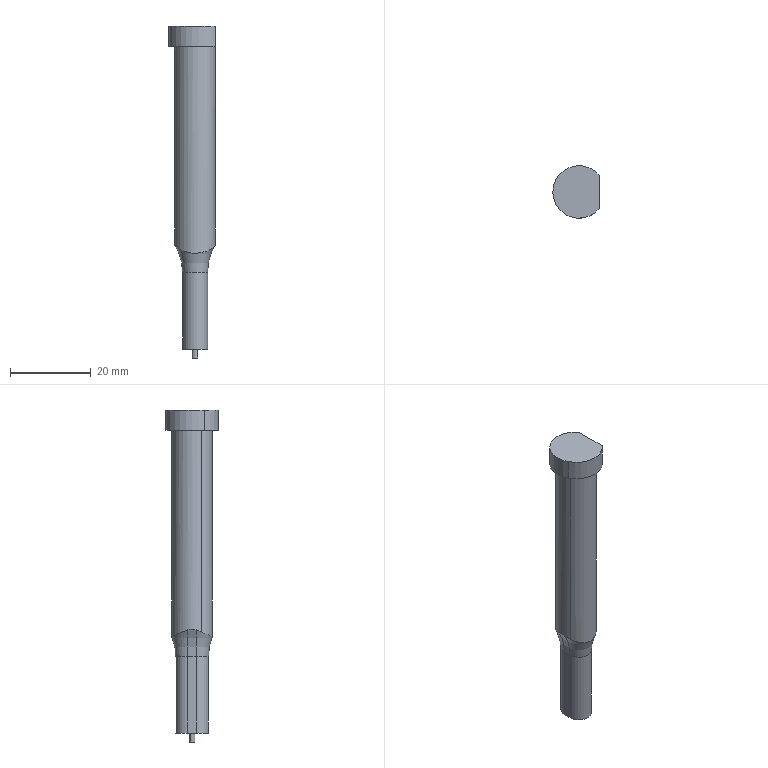Part | CATIA | 1 solid | 19 faces | box 11.5 x 13 x 82.2 mm | volume 5687 mm3 | cylinder 10 | plane 7 | torus 2 | commonest cylinder face diameters 1.47 x2 6.2 x2 10 x2 13 x2 26 x2
STEP:
#1=CARTESIAN_POINT('',(3.1,1.,0.));
#2=VERTEX_POINT('',#1);
#3=CARTESIAN_POINT('',(-3.1,1.,0.));
#4=VERTEX_POINT('',#3);
#5=CARTESIAN_POINT('',(0.,1.,0.));
#6=DIRECTION('',(0.,0.,1.));
#7=AXIS2_PLACEMENT_3D('',#5,#6,$);
#8=CIRCLE('',#7,3.1);
#9=EDGE_CURVE('',#2,#4,#8,.T.);
#10=ORIENTED_EDGE('',*,*,#9,.F.);
#11=CARTESIAN_POINT('',(3.1,-1.,0.));
#12=VERTEX_POINT('',#11);
#13=CARTESIAN_POINT('',(3.1,0.,0.));
#14=DIRECTION('',(0.,-1.,0.));
#15=VECTOR('',#14,1.);
#16=LINE('',#13,#15);
#17=EDGE_CURVE('',#2,#12,#16,.T.);
#18=ORIENTED_EDGE('',*,*,#17,.T.);
#19=CARTESIAN_POINT('',(-3.1,-1.,0.));
#20=VERTEX_POINT('',#19);
#21=CARTESIAN_POINT('',(0.,-1.,0.));
#22=DIRECTION('',(0.,0.,1.));
#23=AXIS2_PLACEMENT_3D('',#21,#22,$);
#24=CIRCLE('',#23,3.1);
#25=EDGE_CURVE('',#20,#12,#24,.T.);
#26=ORIENTED_EDGE('',*,*,#25,.F.);
#27=CARTESIAN_POINT('',(-3.1,0.,0.));
#28=DIRECTION('',(0.,1.,0.));
#29=VECTOR('',#28,1.);
#30=LINE('',#27,#29);
#31=EDGE_CURVE('',#20,#4,#30,.T.);
#32=ORIENTED_EDGE('',*,*,#31,.T.);
#33=EDGE_LOOP('',(#10,#18,#26,#32));
#34=FACE_OUTER_BOUND('',#33,.T.);
#35=CARTESIAN_POINT('',(0.645,-0.3524,0.));
#36=VERTEX_POINT('',#35);
#37=CARTESIAN_POINT('',(-0.645,0.3524,0.));
#38=VERTEX_POINT('',#37);
#39=CARTESIAN_POINT('',(0.,0.,0.));
#40=DIRECTION('',(0.,0.,1.));
#41=AXIS2_PLACEMENT_3D('',#39,#40,$);
#42=CIRCLE('',#41,0.735);
#43=EDGE_CURVE('',#36,#38,#42,.F.);
#44=ORIENTED_EDGE('',*,*,#43,.F.);
#45=CARTESIAN_POINT('',(0.,0.,0.));
#46=DIRECTION('',(0.,0.,1.));
#47=AXIS2_PLACEMENT_3D('',#45,#46,$);
#48=CIRCLE('',#47,0.735);
#49=EDGE_CURVE('',#38,#36,#48,.F.);
#50=ORIENTED_EDGE('',*,*,#49,.F.);
#51=EDGE_LOOP('',(#44,#50));
#52=FACE_BOUND('',#51,.T.);
#53=CARTESIAN_POINT('',(5.,0.,0.));
#54=DIRECTION('',(0.,0.,1.));
#55=DIRECTION('',(1.,0.,0.));
#56=AXIS2_PLACEMENT_3D('',#53,#54,#55);
#57=PLANE('',#56);
#58=ADVANCED_FACE('',(#34,#52),#57,.F.);
#59=CARTESIAN_POINT('',(4.388,2.397,25.072));
#60=VERTEX_POINT('',#59);
#61=CARTESIAN_POINT('',(4.899,1.,25.598));
#62=VERTEX_POINT('',#61);
#63=CARTESIAN_POINT('',(4.388,2.397,25.072));
#64=CARTESIAN_POINT('',(4.62,1.973,25.246));
#65=CARTESIAN_POINT('',(4.797,1.502,25.424));
#66=CARTESIAN_POINT('',(4.899,1.,25.598));
#67=B_SPLINE_CURVE_WITH_KNOTS('',3,(#63,#64,#65,#66),.UNSPECIFIED.,.F.,.U.,(4,4),(0.,5.244),.UNSPECIFIED.);
#68=EDGE_CURVE('',#60,#62,#67,.T.);
#69=ORIENTED_EDGE('',*,*,#68,.F.);
#70=CARTESIAN_POINT('',(4.388,2.397,75.));
#71=VERTEX_POINT('',#70);
#72=CARTESIAN_POINT('',(4.388,2.397,37.5));
#73=DIRECTION('',(0.,0.,1.));
#74=VECTOR('',#73,1.);
#75=LINE('',#72,#74);
#76=EDGE_CURVE('',#60,#71,#75,.T.);
#77=ORIENTED_EDGE('',*,*,#76,.T.);
#78=CARTESIAN_POINT('',(5.,0.,75.));
#79=VERTEX_POINT('',#78);
#80=CARTESIAN_POINT('',(0.,0.,75.));
#81=DIRECTION('',(0.,0.,1.));
#82=AXIS2_PLACEMENT_3D('',#80,#81,$);
#83=CIRCLE('',#82,5.);
#84=EDGE_CURVE('',#79,#71,#83,.T.);
#85=ORIENTED_EDGE('',*,*,#84,.F.);
#86=CARTESIAN_POINT('',(-4.388,-2.397,75.));
#87=VERTEX_POINT('',#86);
#88=CARTESIAN_POINT('',(0.,0.,75.));
#89=DIRECTION('',(0.,0.,1.));
#90=AXIS2_PLACEMENT_3D('',#88,#89,$);
#91=CIRCLE('',#90,5.);
#92=EDGE_CURVE('',#87,#79,#91,.T.);
#93=ORIENTED_EDGE('',*,*,#92,.F.);
#94=CARTESIAN_POINT('',(-4.388,-2.397,25.072));
#95=VERTEX_POINT('',#94);
#96=CARTESIAN_POINT('',(-4.388,-2.397,37.5));
#97=DIRECTION('',(0.,0.,1.));
#98=VECTOR('',#97,1.);
#99=LINE('',#96,#98);
#100=EDGE_CURVE('',#95,#87,#99,.T.);
#101=ORIENTED_EDGE('',*,*,#100,.F.);
#102=CARTESIAN_POINT('',(4.899,-1.,25.598));
#103=VERTEX_POINT('',#102);
#104=CARTESIAN_POINT('',(-4.388,-2.397,25.072));
#105=CARTESIAN_POINT('',(-4.106,-2.913,24.86));
#106=CARTESIAN_POINT('',(-3.757,-3.372,24.653));
#107=CARTESIAN_POINT('',(-3.357,-3.766,24.458));
#108=CARTESIAN_POINT('',(-2.497,-4.411,24.115));
#109=CARTESIAN_POINT('',(-1.535,-4.798,23.881));
#110=CARTESIAN_POINT('',(-1.049,-4.927,23.8));
#111=CARTESIAN_POINT('',(0.1474,-5.089,23.696));
#112=CARTESIAN_POINT('',(1.346,-4.893,23.821));
#113=CARTESIAN_POINT('',(2.03,-4.655,23.973));
#114=CARTESIAN_POINT('',(3.209,-3.988,24.358));
#115=CARTESIAN_POINT('',(4.144,-2.909,24.867));
#116=CARTESIAN_POINT('',(4.498,-2.338,25.111));
#117=CARTESIAN_POINT('',(4.757,-1.693,25.358));
#118=CARTESIAN_POINT('',(4.899,-1.,25.598));
#119=B_SPLINE_CURVE_WITH_KNOTS('',5,(#104,#105,#106,#107,#108,#109,#110,#111,#112,#113,#114,#115,#116,#117,#118),.UNSPECIFIED.,.F.,.U.,(6,3,3,3,6),(0.,10.623,20.893,35.45,47.517),.UNSPECIFIED.);
#120=EDGE_CURVE('',#95,#103,#119,.T.);
#121=ORIENTED_EDGE('',*,*,#120,.T.);
#122=CARTESIAN_POINT('',(4.899,1.,25.598));
#123=CARTESIAN_POINT('',(4.996,0.5243,25.763));
#124=CARTESIAN_POINT('',(5.039,0.000006412,25.828));
#125=CARTESIAN_POINT('',(4.996,-0.5243,25.763));
#126=CARTESIAN_POINT('',(4.899,-1.,25.598));
#127=B_SPLINE_CURVE_WITH_KNOTS('',4,(#122,#123,#124,#125,#126),.UNSPECIFIED.,.F.,.U.,(5,5),(0.,2.9),.UNSPECIFIED.);
#128=EDGE_CURVE('',#62,#103,#127,.T.);
#129=ORIENTED_EDGE('',*,*,#128,.F.);
#130=EDGE_LOOP('',(#69,#77,#85,#93,#101,#121,#129));
#131=FACE_OUTER_BOUND('',#130,.T.);
#132=CARTESIAN_POINT('',(0.,0.,40.));
#133=DIRECTION('',(0.,0.,1.));
#134=DIRECTION('',(0.8776,0.4794,0.));
#135=AXIS2_PLACEMENT_3D('',#132,#133,#134);
#136=CYLINDRICAL_SURFACE('',#135,5.);
#137=ADVANCED_FACE('',(#131),#136,.T.);
#138=CARTESIAN_POINT('',(5.,-4.153,80.));
#139=VERTEX_POINT('',#138);
#140=CARTESIAN_POINT('',(5.,-4.153,75.));
#141=VERTEX_POINT('',#140);
#142=CARTESIAN_POINT('',(5.,-4.153,77.5));
#143=DIRECTION('',(0.,0.,-1.));
#144=VECTOR('',#143,1.);
#145=LINE('',#142,#144);
#146=EDGE_CURVE('',#139,#141,#145,.T.);
#147=ORIENTED_EDGE('',*,*,#146,.T.);
#148=CARTESIAN_POINT('',(5.,-2.077,75.));
#149=DIRECTION('',(0.,-1.,0.));
#150=VECTOR('',#149,1.);
#151=LINE('',#148,#150);
#152=EDGE_CURVE('',#79,#141,#151,.T.);
#153=ORIENTED_EDGE('',*,*,#152,.F.);
#154=CARTESIAN_POINT('',(5.,4.153,75.));
#155=VERTEX_POINT('',#154);
#156=CARTESIAN_POINT('',(5.,2.077,75.));
#157=DIRECTION('',(0.,-1.,0.));
#158=VECTOR('',#157,1.);
#159=LINE('',#156,#158);
#160=EDGE_CURVE('',#155,#79,#159,.T.);
#161=ORIENTED_EDGE('',*,*,#160,.F.);
#162=CARTESIAN_POINT('',(5.,4.153,80.));
#163=VERTEX_POINT('',#162);
#164=CARTESIAN_POINT('',(5.,4.153,77.5));
#165=DIRECTION('',(0.,0.,-1.));
#166=VECTOR('',#165,1.);
#167=LINE('',#164,#166);
#168=EDGE_CURVE('',#163,#155,#167,.T.);
#169=ORIENTED_EDGE('',*,*,#168,.F.);
#170=CARTESIAN_POINT('',(5.,0.,80.));
#171=DIRECTION('',(0.,-1.,0.));
#172=VECTOR('',#171,1.);
#173=LINE('',#170,#172);
#174=EDGE_CURVE('',#163,#139,#173,.T.);
#175=ORIENTED_EDGE('',*,*,#174,.T.);
#176=EDGE_LOOP('',(#147,#153,#161,#169,#175));
#177=FACE_OUTER_BOUND('',#176,.T.);
#178=CARTESIAN_POINT('',(5.,25.,0.));
#179=DIRECTION('',(-1.,0.,0.));
#180=DIRECTION('',(0.,-1.,0.));
#181=AXIS2_PLACEMENT_3D('',#178,#179,#180);
#182=PLANE('',#181);
#183=ADVANCED_FACE('',(#177),#182,.F.);
#184=CARTESIAN_POINT('',(-5.704,-3.116,75.));
#185=VERTEX_POINT('',#184);
#186=CARTESIAN_POINT('',(0.,0.,75.));
#187=DIRECTION('',(0.,0.,1.));
#188=AXIS2_PLACEMENT_3D('',#186,#187,$);
#189=CIRCLE('',#188,6.5);
#190=EDGE_CURVE('',#155,#185,#189,.T.);
#191=ORIENTED_EDGE('',*,*,#190,.T.);
#192=CARTESIAN_POINT('',(-5.704,-3.116,80.));
#193=VERTEX_POINT('',#192);
#194=CARTESIAN_POINT('',(-5.704,-3.116,77.5));
#195=DIRECTION('',(0.,0.,1.));
#196=VECTOR('',#195,1.);
#197=LINE('',#194,#196);
#198=EDGE_CURVE('',#185,#193,#197,.T.);
#199=ORIENTED_EDGE('',*,*,#198,.T.);
#200=CARTESIAN_POINT('',(0.,0.,80.));
#201=DIRECTION('',(0.,0.,1.));
#202=AXIS2_PLACEMENT_3D('',#200,#201,$);
#203=CIRCLE('',#202,6.5);
#204=EDGE_CURVE('',#163,#193,#203,.T.);
#205=ORIENTED_EDGE('',*,*,#204,.F.);
#206=ORIENTED_EDGE('',*,*,#168,.T.);
#207=EDGE_LOOP('',(#191,#199,#205,#206));
#208=FACE_OUTER_BOUND('',#207,.T.);
#209=CARTESIAN_POINT('',(0.,0.,40.));
#210=DIRECTION('',(0.,0.,1.));
#211=DIRECTION('',(0.8776,0.4794,0.));
#212=AXIS2_PLACEMENT_3D('',#209,#210,#211);
#213=CYLINDRICAL_SURFACE('',#212,6.5);
#214=ADVANCED_FACE('',(#208),#213,.T.);
#215=CARTESIAN_POINT('',(0.,0.,80.));
#216=DIRECTION('',(0.,0.,1.));
#217=AXIS2_PLACEMENT_3D('',#215,#216,$);
#218=CIRCLE('',#217,6.5);
#219=EDGE_CURVE('',#193,#139,#218,.T.);
#220=ORIENTED_EDGE('',*,*,#219,.F.);
#221=ORIENTED_EDGE('',*,*,#198,.F.);
#222=CARTESIAN_POINT('',(0.,0.,75.));
#223=DIRECTION('',(0.,0.,1.));
#224=AXIS2_PLACEMENT_3D('',#222,#223,$);
#225=CIRCLE('',#224,6.5);
#226=EDGE_CURVE('',#185,#141,#225,.T.);
#227=ORIENTED_EDGE('',*,*,#226,.T.);
#228=ORIENTED_EDGE('',*,*,#146,.F.);
#229=EDGE_LOOP('',(#220,#221,#227,#228));
#230=FACE_OUTER_BOUND('',#229,.T.);
#231=ADVANCED_FACE('',(#230),#213,.T.);
#232=ORIENTED_EDGE('',*,*,#160,.T.);
#233=ORIENTED_EDGE('',*,*,#84,.T.);
#234=CARTESIAN_POINT('',(0.,0.,75.));
#235=DIRECTION('',(0.,0.,1.));
#236=AXIS2_PLACEMENT_3D('',#234,#235,$);
#237=CIRCLE('',#236,5.);
#238=EDGE_CURVE('',#71,#87,#237,.T.);
#239=ORIENTED_EDGE('',*,*,#238,.T.);
#240=ORIENTED_EDGE('',*,*,#92,.T.);
#241=ORIENTED_EDGE('',*,*,#152,.T.);
#242=ORIENTED_EDGE('',*,*,#226,.F.);
#243=ORIENTED_EDGE('',*,*,#190,.F.);
#244=EDGE_LOOP('',(#232,#233,#239,#240,#241,#242,#243));
#245=FACE_OUTER_BOUND('',#244,.T.);
#246=CARTESIAN_POINT('',(6.5,0.,75.));
#247=DIRECTION('',(0.,0.,1.));
#248=DIRECTION('',(1.,0.,0.));
#249=AXIS2_PLACEMENT_3D('',#246,#247,#248);
#250=PLANE('',#249);
#251=ADVANCED_FACE('',(#245),#250,.F.);
#252=ORIENTED_EDGE('',*,*,#204,.T.);
#253=ORIENTED_EDGE('',*,*,#219,.T.);
#254=ORIENTED_EDGE('',*,*,#174,.F.);
#255=EDGE_LOOP('',(#252,#253,#254));
#256=FACE_OUTER_BOUND('',#255,.T.);
#257=CARTESIAN_POINT('',(0.,0.,80.));
#258=DIRECTION('',(0.,0.,1.));
#259=DIRECTION('',(1.,0.,0.));
#260=AXIS2_PLACEMENT_3D('',#257,#258,#259);
#261=PLANE('',#260);
#262=ADVANCED_FACE('',(#256),#261,.T.);
#263=ORIENTED_EDGE('',*,*,#128,.T.);
#264=CARTESIAN_POINT('',(3.1,-1.,19.));
#265=VERTEX_POINT('',#264);
#266=CARTESIAN_POINT('',(16.1,-1.,19.));
#267=DIRECTION('',(0.,-1.,0.));
#268=AXIS2_PLACEMENT_3D('',#266,#267,$);
#269=CIRCLE('',#268,13.);
#270=EDGE_CURVE('',#103,#265,#269,.T.);
#271=ORIENTED_EDGE('',*,*,#270,.T.);
#272=CARTESIAN_POINT('',(3.1,1.,19.));
#273=VERTEX_POINT('',#272);
#274=CARTESIAN_POINT('',(3.1,0.,19.));
#275=DIRECTION('',(0.,-1.,0.));
#276=VECTOR('',#275,1.);
#277=LINE('',#274,#276);
#278=EDGE_CURVE('',#273,#265,#277,.T.);
#279=ORIENTED_EDGE('',*,*,#278,.F.);
#280=CARTESIAN_POINT('',(16.1,1.,19.));
#281=DIRECTION('',(0.,-1.,0.));
#282=AXIS2_PLACEMENT_3D('',#280,#281,$);
#283=CIRCLE('',#282,13.);
#284=EDGE_CURVE('',#62,#273,#283,.T.);
#285=ORIENTED_EDGE('',*,*,#284,.F.);
#286=EDGE_LOOP('',(#263,#271,#279,#285));
#287=FACE_OUTER_BOUND('',#286,.T.);
#288=CARTESIAN_POINT('',(16.1,0.,19.));
#289=DIRECTION('',(0.,-1.,0.));
#290=DIRECTION('',(0.,0.,1.));
#291=AXIS2_PLACEMENT_3D('',#288,#289,#290);
#292=CYLINDRICAL_SURFACE('',#291,13.);
#293=ADVANCED_FACE('',(#287),#292,.F.);
#294=CARTESIAN_POINT('',(-4.899,1.,25.598));
#295=VERTEX_POINT('',#294);
#296=CARTESIAN_POINT('',(4.388,2.397,25.072));
#297=CARTESIAN_POINT('',(4.106,2.913,24.86));
#298=CARTESIAN_POINT('',(3.757,3.372,24.653));
#299=CARTESIAN_POINT('',(3.357,3.766,24.458));
#300=CARTESIAN_POINT('',(2.497,4.411,24.115));
#301=CARTESIAN_POINT('',(1.535,4.798,23.881));
#302=CARTESIAN_POINT('',(1.049,4.927,23.8));
#303=CARTESIAN_POINT('',(-0.1474,5.089,23.696));
#304=CARTESIAN_POINT('',(-1.346,4.893,23.821));
#305=CARTESIAN_POINT('',(-2.03,4.655,23.973));
#306=CARTESIAN_POINT('',(-3.209,3.988,24.358));
#307=CARTESIAN_POINT('',(-4.144,2.909,24.867));
#308=CARTESIAN_POINT('',(-4.498,2.338,25.111));
#309=CARTESIAN_POINT('',(-4.757,1.693,25.358));
#310=CARTESIAN_POINT('',(-4.899,1.,25.598));
#311=B_SPLINE_CURVE_WITH_KNOTS('',5,(#296,#297,#298,#299,#300,#301,#302,#303,#304,#305,#306,#307,#308,#309,#310),.UNSPECIFIED.,.F.,.U.,(6,3,3,3,6),(0.,10.623,20.893,35.45,47.517),.UNSPECIFIED.);
#312=EDGE_CURVE('',#60,#295,#311,.T.);
#313=ORIENTED_EDGE('',*,*,#312,.F.);
#314=ORIENTED_EDGE('',*,*,#68,.T.);
#315=ORIENTED_EDGE('',*,*,#284,.T.);
#316=CARTESIAN_POINT('',(-3.1,1.,19.));
#317=VERTEX_POINT('',#316);
#318=CARTESIAN_POINT('',(0.,1.,19.));
#319=DIRECTION('',(0.,0.,-1.));
#320=AXIS2_PLACEMENT_3D('',#318,#319,$);
#321=CIRCLE('',#320,3.1);
#322=EDGE_CURVE('',#317,#273,#321,.T.);
#323=ORIENTED_EDGE('',*,*,#322,.F.);
#324=CARTESIAN_POINT('',(-16.1,1.,19.));
#325=DIRECTION('',(0.,-1.,0.));
#326=AXIS2_PLACEMENT_3D('',#324,#325,$);
#327=CIRCLE('',#326,13.);
#328=EDGE_CURVE('',#295,#317,#327,.F.);
#329=ORIENTED_EDGE('',*,*,#328,.F.);
#330=EDGE_LOOP('',(#313,#314,#315,#323,#329));
#331=FACE_OUTER_BOUND('',#330,.T.);
#332=CARTESIAN_POINT('',(0.,1.,19.));
#333=DIRECTION('',(0.,0.,-1.));
#334=DIRECTION('',(-0.9734,-0.2293,0.));
#335=AXIS2_PLACEMENT_3D('',#332,#333,#334);
#336=TOROIDAL_SURFACE('',#335,16.1,13.);
#337=ADVANCED_FACE('',(#331),#336,.F.);
#338=ORIENTED_EDGE('',*,*,#120,.F.);
#339=CARTESIAN_POINT('',(-4.899,-1.,25.598));
#340=VERTEX_POINT('',#339);
#341=CARTESIAN_POINT('',(-4.388,-2.397,25.072));
#342=CARTESIAN_POINT('',(-4.62,-1.973,25.246));
#343=CARTESIAN_POINT('',(-4.797,-1.502,25.424));
#344=CARTESIAN_POINT('',(-4.899,-1.,25.598));
#345=B_SPLINE_CURVE_WITH_KNOTS('',3,(#341,#342,#343,#344),.UNSPECIFIED.,.F.,.U.,(4,4),(0.,5.244),.UNSPECIFIED.);
#346=EDGE_CURVE('',#95,#340,#345,.T.);
#347=ORIENTED_EDGE('',*,*,#346,.T.);
#348=CARTESIAN_POINT('',(-3.1,-1.,19.));
#349=VERTEX_POINT('',#348);
#350=CARTESIAN_POINT('',(-16.1,-1.,19.));
#351=DIRECTION('',(0.,-1.,0.));
#352=AXIS2_PLACEMENT_3D('',#350,#351,$);
#353=CIRCLE('',#352,13.);
#354=EDGE_CURVE('',#340,#349,#353,.F.);
#355=ORIENTED_EDGE('',*,*,#354,.T.);
#356=CARTESIAN_POINT('',(0.,-1.,19.));
#357=DIRECTION('',(0.,0.,-1.));
#358=AXIS2_PLACEMENT_3D('',#356,#357,$);
#359=CIRCLE('',#358,3.1);
#360=EDGE_CURVE('',#265,#349,#359,.T.);
#361=ORIENTED_EDGE('',*,*,#360,.F.);
#362=ORIENTED_EDGE('',*,*,#270,.F.);
#363=EDGE_LOOP('',(#338,#347,#355,#361,#362));
#364=FACE_OUTER_BOUND('',#363,.T.);
#365=CARTESIAN_POINT('',(0.,-1.,19.));
#366=DIRECTION('',(0.,0.,-1.));
#367=DIRECTION('',(0.9862,0.1654,0.));
#368=AXIS2_PLACEMENT_3D('',#365,#366,#367);
#369=TOROIDAL_SURFACE('',#368,16.1,13.);
#370=ADVANCED_FACE('',(#364),#369,.F.);
#371=ORIENTED_EDGE('',*,*,#278,.T.);
#372=CARTESIAN_POINT('',(3.1,-1.,9.5));
#373=DIRECTION('',(0.,0.,1.));
#374=VECTOR('',#373,1.);
#375=LINE('',#372,#374);
#376=EDGE_CURVE('',#12,#265,#375,.T.);
#377=ORIENTED_EDGE('',*,*,#376,.F.);
#378=ORIENTED_EDGE('',*,*,#17,.F.);
#379=CARTESIAN_POINT('',(3.1,1.,9.5));
#380=DIRECTION('',(0.,0.,1.));
#381=VECTOR('',#380,1.);
#382=LINE('',#379,#381);
#383=EDGE_CURVE('',#2,#273,#382,.T.);
#384=ORIENTED_EDGE('',*,*,#383,.T.);
#385=EDGE_LOOP('',(#371,#377,#378,#384));
#386=FACE_OUTER_BOUND('',#385,.T.);
#387=CARTESIAN_POINT('',(3.1,1.,0.));
#388=DIRECTION('',(-1.,0.,0.));
#389=DIRECTION('',(0.,-1.,0.));
#390=AXIS2_PLACEMENT_3D('',#387,#388,#389);
#391=PLANE('',#390);
#392=ADVANCED_FACE('',(#386),#391,.F.);
#393=CARTESIAN_POINT('',(-4.899,-1.,25.598));
#394=CARTESIAN_POINT('',(-4.996,-0.5243,25.763));
#395=CARTESIAN_POINT('',(-5.039,-0.000006352,25.828));
#396=CARTESIAN_POINT('',(-4.996,0.5243,25.763));
#397=CARTESIAN_POINT('',(-4.899,1.,25.598));
#398=B_SPLINE_CURVE_WITH_KNOTS('',4,(#393,#394,#395,#396,#397),.UNSPECIFIED.,.F.,.U.,(5,5),(0.,2.9),.UNSPECIFIED.);
#399=EDGE_CURVE('',#340,#295,#398,.T.);
#400=ORIENTED_EDGE('',*,*,#399,.T.);
#401=ORIENTED_EDGE('',*,*,#328,.T.);
#402=CARTESIAN_POINT('',(-3.1,0.,19.));
#403=DIRECTION('',(0.,1.,0.));
#404=VECTOR('',#403,1.);
#405=LINE('',#402,#404);
#406=EDGE_CURVE('',#349,#317,#405,.T.);
#407=ORIENTED_EDGE('',*,*,#406,.F.);
#408=ORIENTED_EDGE('',*,*,#354,.F.);
#409=EDGE_LOOP('',(#400,#401,#407,#408));
#410=FACE_OUTER_BOUND('',#409,.T.);
#411=CARTESIAN_POINT('',(-16.1,0.,19.));
#412=DIRECTION('',(0.,1.,0.));
#413=DIRECTION('',(0.,0.,1.));
#414=AXIS2_PLACEMENT_3D('',#411,#412,#413);
#415=CYLINDRICAL_SURFACE('',#414,13.);
#416=ADVANCED_FACE('',(#410),#415,.F.);
#417=ORIENTED_EDGE('',*,*,#383,.F.);
#418=ORIENTED_EDGE('',*,*,#9,.T.);
#419=CARTESIAN_POINT('',(-3.1,1.,16.61));
#420=DIRECTION('',(0.,0.,1.));
#421=VECTOR('',#420,1.);
#422=LINE('',#419,#421);
#423=EDGE_CURVE('',#4,#317,#422,.T.);
#424=ORIENTED_EDGE('',*,*,#423,.T.);
#425=ORIENTED_EDGE('',*,*,#322,.T.);
#426=EDGE_LOOP('',(#417,#418,#424,#425));
#427=FACE_OUTER_BOUND('',#426,.T.);
#428=CARTESIAN_POINT('',(0.,1.,16.61));
#429=DIRECTION('',(0.,0.,1.));
#430=DIRECTION('',(1.,0.,0.));
#431=AXIS2_PLACEMENT_3D('',#428,#429,#430);
#432=CYLINDRICAL_SURFACE('',#431,3.1);
#433=ADVANCED_FACE('',(#427),#432,.T.);
#434=CARTESIAN_POINT('',(-3.1,-1.,16.61));
#435=DIRECTION('',(0.,0.,1.));
#436=VECTOR('',#435,1.);
#437=LINE('',#434,#436);
#438=EDGE_CURVE('',#20,#349,#437,.T.);
#439=ORIENTED_EDGE('',*,*,#438,.F.);
#440=ORIENTED_EDGE('',*,*,#25,.T.);
#441=ORIENTED_EDGE('',*,*,#376,.T.);
#442=ORIENTED_EDGE('',*,*,#360,.T.);
#443=EDGE_LOOP('',(#439,#440,#441,#442));
#444=FACE_OUTER_BOUND('',#443,.T.);
#445=CARTESIAN_POINT('',(0.,-1.,16.61));
#446=DIRECTION('',(0.,0.,1.));
#447=DIRECTION('',(-1.,0.,0.));
#448=AXIS2_PLACEMENT_3D('',#445,#446,#447);
#449=CYLINDRICAL_SURFACE('',#448,3.1);
#450=ADVANCED_FACE('',(#444),#449,.T.);
#451=ORIENTED_EDGE('',*,*,#406,.T.);
#452=ORIENTED_EDGE('',*,*,#423,.F.);
#453=ORIENTED_EDGE('',*,*,#31,.F.);
#454=ORIENTED_EDGE('',*,*,#438,.T.);
#455=EDGE_LOOP('',(#451,#452,#453,#454));
#456=FACE_OUTER_BOUND('',#455,.T.);
#457=CARTESIAN_POINT('',(-3.1,-1.,0.));
#458=DIRECTION('',(1.,0.,0.));
#459=DIRECTION('',(0.,1.,0.));
#460=AXIS2_PLACEMENT_3D('',#457,#458,#459);
#461=PLANE('',#460);
#462=ADVANCED_FACE('',(#456),#461,.F.);
#463=ORIENTED_EDGE('',*,*,#100,.T.);
#464=ORIENTED_EDGE('',*,*,#238,.F.);
#465=ORIENTED_EDGE('',*,*,#76,.F.);
#466=ORIENTED_EDGE('',*,*,#312,.T.);
#467=ORIENTED_EDGE('',*,*,#399,.F.);
#468=ORIENTED_EDGE('',*,*,#346,.F.);
#469=EDGE_LOOP('',(#463,#464,#465,#466,#467,#468));
#470=FACE_OUTER_BOUND('',#469,.T.);
#471=ADVANCED_FACE('',(#470),#136,.T.);
#472=CARTESIAN_POINT('',(0.645,-0.3524,-2.2));
#473=VERTEX_POINT('',#472);
#474=CARTESIAN_POINT('',(-0.645,0.3524,-2.2));
#475=VERTEX_POINT('',#474);
#476=CARTESIAN_POINT('',(0.,0.,-2.2));
#477=DIRECTION('',(0.,0.,-1.));
#478=AXIS2_PLACEMENT_3D('',#476,#477,$);
#479=CIRCLE('',#478,0.735);
#480=EDGE_CURVE('',#473,#475,#479,.T.);
#481=ORIENTED_EDGE('',*,*,#480,.F.);
#482=CARTESIAN_POINT('',(0.645,-0.3524,-1.1));
#483=DIRECTION('',(0.,0.,-1.));
#484=VECTOR('',#483,1.);
#485=LINE('',#482,#484);
#486=EDGE_CURVE('',#473,#36,#485,.F.);
#487=ORIENTED_EDGE('',*,*,#486,.T.);
#488=ORIENTED_EDGE('',*,*,#43,.T.);
#489=CARTESIAN_POINT('',(-0.645,0.3524,-1.1));
#490=DIRECTION('',(0.,0.,-1.));
#491=VECTOR('',#490,1.);
#492=LINE('',#489,#491);
#493=EDGE_CURVE('',#475,#38,#492,.F.);
#494=ORIENTED_EDGE('',*,*,#493,.F.);
#495=EDGE_LOOP('',(#481,#487,#488,#494));
#496=FACE_OUTER_BOUND('',#495,.T.);
#497=CARTESIAN_POINT('',(0.,0.,-1.1));
#498=DIRECTION('',(0.,0.,-1.));
#499=DIRECTION('',(0.8776,-0.4794,0.));
#500=AXIS2_PLACEMENT_3D('',#497,#498,#499);
#501=CYLINDRICAL_SURFACE('',#500,0.735);
#502=ADVANCED_FACE('',(#496),#501,.T.);
#503=CARTESIAN_POINT('',(0.,0.,-2.2));
#504=DIRECTION('',(0.,0.,-1.));
#505=AXIS2_PLACEMENT_3D('',#503,#504,$);
#506=CIRCLE('',#505,0.735);
#507=EDGE_CURVE('',#475,#473,#506,.T.);
#508=ORIENTED_EDGE('',*,*,#507,.F.);
#509=ORIENTED_EDGE('',*,*,#493,.T.);
#510=ORIENTED_EDGE('',*,*,#49,.T.);
#511=ORIENTED_EDGE('',*,*,#486,.F.);
#512=EDGE_LOOP('',(#508,#509,#510,#511));
#513=FACE_OUTER_BOUND('',#512,.T.);
#514=ADVANCED_FACE('',(#513),#501,.T.);
#515=ORIENTED_EDGE('',*,*,#480,.T.);
#516=ORIENTED_EDGE('',*,*,#507,.T.);
#517=EDGE_LOOP('',(#515,#516));
#518=FACE_OUTER_BOUND('',#517,.T.);
#519=CARTESIAN_POINT('',(0.735,0.,-2.2));
#520=DIRECTION('',(0.,0.,-1.));
#521=DIRECTION('',(1.,0.,0.));
#522=AXIS2_PLACEMENT_3D('',#519,#520,#521);
#523=PLANE('',#522);
#524=ADVANCED_FACE('',(#518),#523,.T.);
#525=CLOSED_SHELL('',(#58,#137,#183,#214,#231,#251,#262,#293,#337,#370,#392,#416,#433,#450,#462,#471,#502,#514,#524));
#526=MANIFOLD_SOLID_BREP('',#525);
#527=(LENGTH_UNIT()NAMED_UNIT(*)SI_UNIT(.MILLI.,.METRE.));
#528=UNCERTAINTY_MEASURE_WITH_UNIT(LENGTH_MEASURE(0.005),#527,'','');
#529=(NAMED_UNIT(*)PLANE_ANGLE_UNIT()SI_UNIT($,.RADIAN.));
#530=(NAMED_UNIT(*)SI_UNIT($,.STERADIAN.)SOLID_ANGLE_UNIT());
#531=(GEOMETRIC_REPRESENTATION_CONTEXT(3)GLOBAL_UNCERTAINTY_ASSIGNED_CONTEXT((#528))GLOBAL_UNIT_ASSIGNED_CONTEXT((#527,#529,#530))REPRESENTATION_CONTEXT('',''));
#532=ADVANCED_BREP_SHAPE_REPRESENTATION('',(#526),#531);